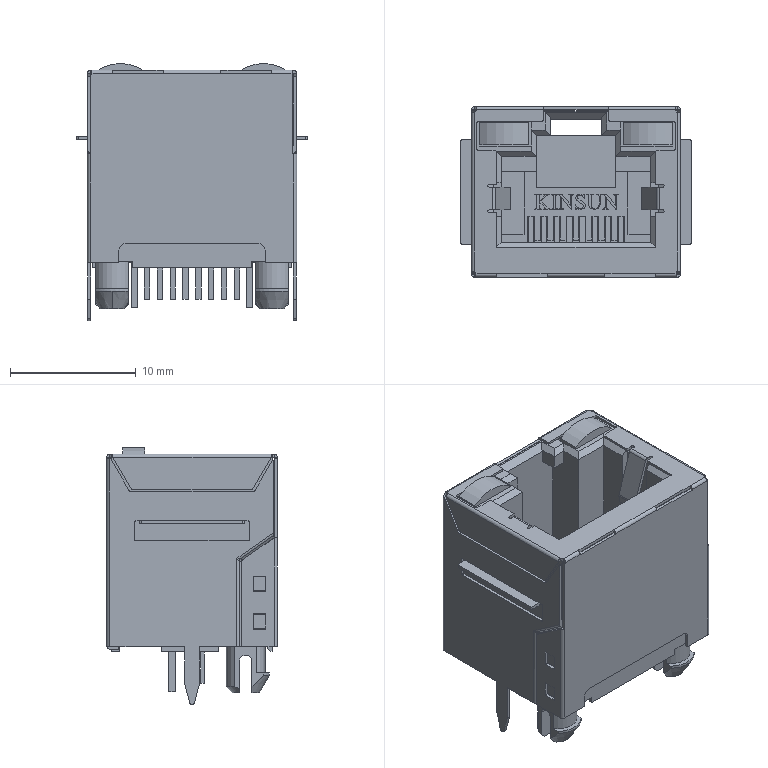Part | SolidWorks | features BaseBody 1 | 1 solid | 1134 faces | box 18.3 x 13.55 x 20.425 mm | volume 1911 mm3 | plane 827 | cylinder 240 | spline 62 | cone 5 | commonest cylinder face diameters 0.5 x59 1 x30 0.4 x29 0.2 x22 0.85 x16 1.45 x16